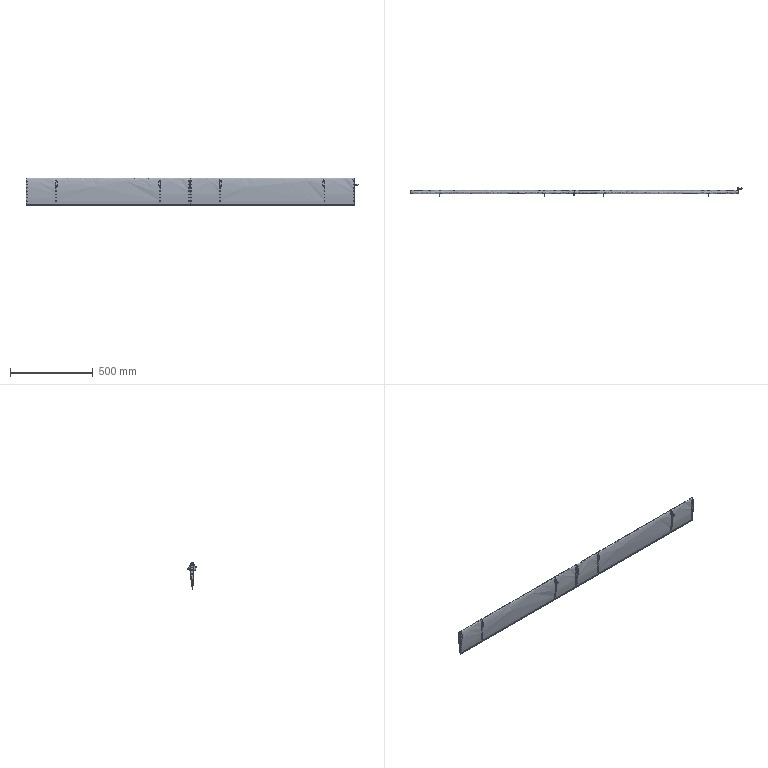Part | SolidWorks | features BaseBody 33 | 33 solids | 1103 faces | box 2003 x 52.2 x 165.107 mm | volume 654070 mm3 | cylinder 662 | plane 275 | spline 148 | cone 18 | commonest cylinder face diameters 3.2 x504 5 x48 3 x32 12 x28 2.614 x16 2.827 x8